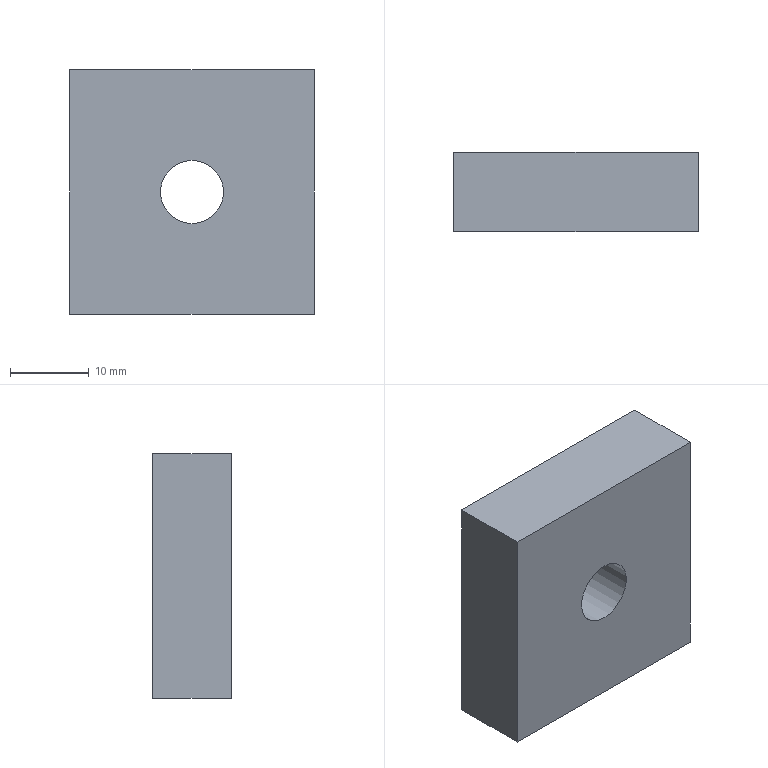Part | STEP file | solid 209 | 1 solid | 7 faces | box 31 x 10 x 31 mm | volume 9107 mm3 | plane 6 | cylinder 1 | commonest cylinder face diameters 8 x1